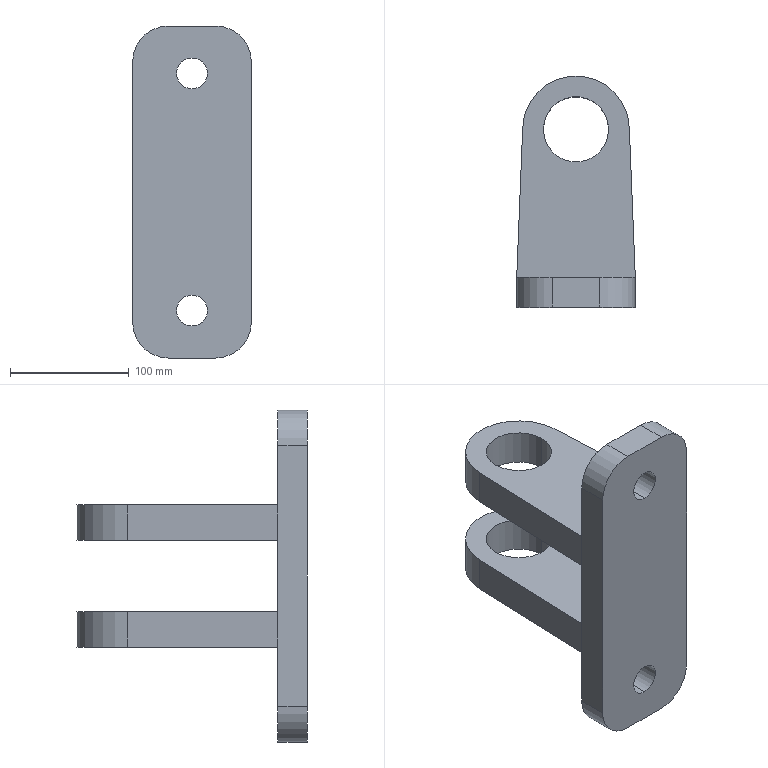Part | SolidWorks | features ICE 3, Extrusion 1, Fillet 1, MirrorPattern 1 | 1 solid | 30 faces | box 100 x 195 x 280 mm | volume 1415210 mm3 | plane 16 | cylinder 14 | commonest cylinder face diameters 26 x4 55 x4 60 x4 90 x2
STEP:
#1=CARTESIAN_POINT('',(0.,25.,87.));
#2=VERTEX_POINT('',#1);
#3=CARTESIAN_POINT('',(0.,25.,113.));
#4=VERTEX_POINT('',#3);
#5=CARTESIAN_POINT('',(0.,25.,100.));
#6=DIRECTION('',(0.,1.,0.));
#7=DIRECTION('',(0.,0.,-1.));
#8=AXIS2_PLACEMENT_3D('',#5,#6,#7);
#9=CIRCLE('',#8,13.);
#10=EDGE_CURVE('',#2,#4,#9,.T.);
#11=ORIENTED_EDGE('',*,*,#10,.T.);
#12=CARTESIAN_POINT('',(0.,0.,113.));
#13=VERTEX_POINT('',#12);
#14=CARTESIAN_POINT('',(0.,322.321,113.));
#15=DIRECTION('',(0.,-1.,0.));
#16=VECTOR('',#15,1000.);
#17=LINE('',#14,#16);
#18=EDGE_CURVE('',#4,#13,#17,.T.);
#19=ORIENTED_EDGE('',*,*,#18,.T.);
#20=CARTESIAN_POINT('',(0.,0.,87.));
#21=VERTEX_POINT('',#20);
#22=CARTESIAN_POINT('',(0.,0.,100.));
#23=DIRECTION('',(0.,-1.,0.));
#24=DIRECTION('',(0.,0.,1.));
#25=AXIS2_PLACEMENT_3D('',#22,#23,#24);
#26=CIRCLE('',#25,13.);
#27=EDGE_CURVE('',#13,#21,#26,.T.);
#28=ORIENTED_EDGE('',*,*,#27,.T.);
#29=CARTESIAN_POINT('',(0.,322.321,87.));
#30=DIRECTION('',(0.,-1.,0.));
#31=VECTOR('',#30,1000.);
#32=LINE('',#29,#31);
#33=EDGE_CURVE('',#2,#21,#32,.T.);
#34=ORIENTED_EDGE('',*,*,#33,.F.);
#35=EDGE_LOOP('',(#11,#19,#28,#34));
#36=FACE_OUTER_BOUND('',#35,.T.);
#37=CARTESIAN_POINT('',(0.,322.321,100.));
#38=DIRECTION('',(0.,-1.,0.));
#39=DIRECTION('',(0.,0.,-1.));
#40=AXIS2_PLACEMENT_3D('',#37,#38,#39);
#41=CYLINDRICAL_SURFACE('',#40,13.);
#42=ADVANCED_FACE('',(#36),#41,.F.);
#43=CARTESIAN_POINT('',(0.,25.,-113.));
#44=VERTEX_POINT('',#43);
#45=CARTESIAN_POINT('',(0.,25.,-87.));
#46=VERTEX_POINT('',#45);
#47=CARTESIAN_POINT('',(0.,25.,-100.));
#48=DIRECTION('',(0.,1.,0.));
#49=DIRECTION('',(0.,0.,-1.));
#50=AXIS2_PLACEMENT_3D('',#47,#48,#49);
#51=CIRCLE('',#50,13.);
#52=EDGE_CURVE('',#44,#46,#51,.T.);
#53=ORIENTED_EDGE('',*,*,#52,.T.);
#54=CARTESIAN_POINT('',(0.,0.,-87.));
#55=VERTEX_POINT('',#54);
#56=CARTESIAN_POINT('',(0.,322.321,-87.));
#57=DIRECTION('',(0.,-1.,0.));
#58=VECTOR('',#57,1000.);
#59=LINE('',#56,#58);
#60=EDGE_CURVE('',#46,#55,#59,.T.);
#61=ORIENTED_EDGE('',*,*,#60,.T.);
#62=CARTESIAN_POINT('',(0.,0.,-113.));
#63=VERTEX_POINT('',#62);
#64=CARTESIAN_POINT('',(0.,0.,-100.));
#65=DIRECTION('',(0.,-1.,0.));
#66=DIRECTION('',(0.,0.,-1.));
#67=AXIS2_PLACEMENT_3D('',#64,#65,#66);
#68=CIRCLE('',#67,13.);
#69=EDGE_CURVE('',#55,#63,#68,.T.);
#70=ORIENTED_EDGE('',*,*,#69,.T.);
#71=CARTESIAN_POINT('',(0.,322.321,-113.));
#72=DIRECTION('',(0.,-1.,0.));
#73=VECTOR('',#72,1000.);
#74=LINE('',#71,#73);
#75=EDGE_CURVE('',#44,#63,#74,.T.);
#76=ORIENTED_EDGE('',*,*,#75,.F.);
#77=EDGE_LOOP('',(#53,#61,#70,#76));
#78=FACE_OUTER_BOUND('',#77,.T.);
#79=CARTESIAN_POINT('',(0.,322.321,-100.));
#80=DIRECTION('',(0.,-1.,0.));
#81=DIRECTION('',(0.,0.,-1.));
#82=AXIS2_PLACEMENT_3D('',#79,#80,#81);
#83=CYLINDRICAL_SURFACE('',#82,13.);
#84=ADVANCED_FACE('',(#78),#83,.F.);
#85=CARTESIAN_POINT('',(-27.5,150.,-30.));
#86=VERTEX_POINT('',#85);
#87=CARTESIAN_POINT('',(27.5,150.,-30.));
#88=VERTEX_POINT('',#87);
#89=CARTESIAN_POINT('',(0.,150.,-30.));
#90=DIRECTION('',(0.,0.,1.));
#91=DIRECTION('',(1.,0.,0.));
#92=AXIS2_PLACEMENT_3D('',#89,#90,#91);
#93=CIRCLE('',#92,27.5);
#94=EDGE_CURVE('',#86,#88,#93,.T.);
#95=ORIENTED_EDGE('',*,*,#94,.T.);
#96=CARTESIAN_POINT('',(27.5,150.,-60.));
#97=VERTEX_POINT('',#96);
#98=CARTESIAN_POINT('',(27.5,150.,-30.));
#99=DIRECTION('',(0.,0.,-1.));
#100=VECTOR('',#99,1000.);
#101=LINE('',#98,#100);
#102=EDGE_CURVE('',#88,#97,#101,.T.);
#103=ORIENTED_EDGE('',*,*,#102,.T.);
#104=CARTESIAN_POINT('',(-27.5,150.,-60.));
#105=VERTEX_POINT('',#104);
#106=CARTESIAN_POINT('',(0.,150.,-60.));
#107=DIRECTION('',(0.,0.,1.));
#108=DIRECTION('',(1.,0.,0.));
#109=AXIS2_PLACEMENT_3D('',#106,#107,#108);
#110=CIRCLE('',#109,27.5);
#111=EDGE_CURVE('',#105,#97,#110,.T.);
#112=ORIENTED_EDGE('',*,*,#111,.F.);
#113=CARTESIAN_POINT('',(-27.5,150.,-30.));
#114=DIRECTION('',(0.,0.,-1.));
#115=VECTOR('',#114,1000.);
#116=LINE('',#113,#115);
#117=EDGE_CURVE('',#86,#105,#116,.T.);
#118=ORIENTED_EDGE('',*,*,#117,.F.);
#119=EDGE_LOOP('',(#95,#103,#112,#118));
#120=FACE_OUTER_BOUND('',#119,.T.);
#121=CARTESIAN_POINT('',(0.,150.,-30.));
#122=DIRECTION('',(0.,0.,-1.));
#123=DIRECTION('',(-1.,0.,0.));
#124=AXIS2_PLACEMENT_3D('',#121,#122,#123);
#125=CYLINDRICAL_SURFACE('',#124,27.5);
#126=ADVANCED_FACE('',(#120),#125,.F.);
#127=CARTESIAN_POINT('',(-27.5,150.,30.));
#128=VERTEX_POINT('',#127);
#129=CARTESIAN_POINT('',(27.5,150.,30.));
#130=VERTEX_POINT('',#129);
#131=CARTESIAN_POINT('',(0.,150.,30.));
#132=DIRECTION('',(0.,0.,1.));
#133=DIRECTION('',(1.,0.,0.));
#134=AXIS2_PLACEMENT_3D('',#131,#132,#133);
#135=CIRCLE('',#134,27.5);
#136=EDGE_CURVE('',#128,#130,#135,.T.);
#137=ORIENTED_EDGE('',*,*,#136,.F.);
#138=CARTESIAN_POINT('',(-27.5,150.,60.));
#139=VERTEX_POINT('',#138);
#140=CARTESIAN_POINT('',(-27.5,150.,30.));
#141=DIRECTION('',(0.,0.,1.));
#142=VECTOR('',#141,1000.);
#143=LINE('',#140,#142);
#144=EDGE_CURVE('',#128,#139,#143,.T.);
#145=ORIENTED_EDGE('',*,*,#144,.T.);
#146=CARTESIAN_POINT('',(27.5,150.,60.));
#147=VERTEX_POINT('',#146);
#148=CARTESIAN_POINT('',(0.,150.,60.));
#149=DIRECTION('',(0.,0.,1.));
#150=DIRECTION('',(1.,0.,0.));
#151=AXIS2_PLACEMENT_3D('',#148,#149,#150);
#152=CIRCLE('',#151,27.5);
#153=EDGE_CURVE('',#139,#147,#152,.T.);
#154=ORIENTED_EDGE('',*,*,#153,.T.);
#155=CARTESIAN_POINT('',(27.5,150.,30.));
#156=DIRECTION('',(0.,0.,1.));
#157=VECTOR('',#156,1000.);
#158=LINE('',#155,#157);
#159=EDGE_CURVE('',#130,#147,#158,.T.);
#160=ORIENTED_EDGE('',*,*,#159,.F.);
#161=EDGE_LOOP('',(#137,#145,#154,#160));
#162=FACE_OUTER_BOUND('',#161,.T.);
#163=CARTESIAN_POINT('',(0.,150.,30.));
#164=DIRECTION('',(0.,0.,1.));
#165=DIRECTION('',(1.,0.,0.));
#166=AXIS2_PLACEMENT_3D('',#163,#164,#165);
#167=CYLINDRICAL_SURFACE('',#166,27.5);
#168=ADVANCED_FACE('',(#162),#167,.F.);
#169=CARTESIAN_POINT('',(0.,150.,60.));
#170=DIRECTION('',(0.,0.,1.));
#171=DIRECTION('',(1.,0.,0.));
#172=AXIS2_PLACEMENT_3D('',#169,#170,#171);
#173=CIRCLE('',#172,27.5);
#174=EDGE_CURVE('',#147,#139,#173,.T.);
#175=ORIENTED_EDGE('',*,*,#174,.F.);
#176=ORIENTED_EDGE('',*,*,#153,.F.);
#177=EDGE_LOOP('',(#175,#176));
#178=FACE_BOUND('',#177,.T.);
#179=CARTESIAN_POINT('',(50.,25.,60.));
#180=VERTEX_POINT('',#179);
#181=CARTESIAN_POINT('',(-50.,25.,60.));
#182=VERTEX_POINT('',#181);
#183=CARTESIAN_POINT('',(-7.5,25.,60.));
#184=DIRECTION('',(-1.,0.,0.));
#185=VECTOR('',#184,1000.);
#186=LINE('',#183,#185);
#187=EDGE_CURVE('',#180,#182,#186,.T.);
#188=ORIENTED_EDGE('',*,*,#187,.F.);
#189=CARTESIAN_POINT('',(44.965,151.786,60.));
#190=VERTEX_POINT('',#189);
#191=CARTESIAN_POINT('',(44.965,151.786,60.));
#192=DIRECTION('',(-0.03968,0.9992,0.));
#193=VECTOR('',#192,1000.);
#194=LINE('',#191,#193);
#195=EDGE_CURVE('',#180,#190,#194,.T.);
#196=ORIENTED_EDGE('',*,*,#195,.T.);
#197=CARTESIAN_POINT('',(-44.965,151.786,60.));
#198=VERTEX_POINT('',#197);
#199=CARTESIAN_POINT('',(0.,150.,60.));
#200=DIRECTION('',(0.,0.,1.));
#201=DIRECTION('',(1.,0.,0.));
#202=AXIS2_PLACEMENT_3D('',#199,#200,#201);
#203=CIRCLE('',#202,45.);
#204=EDGE_CURVE('',#190,#198,#203,.T.);
#205=ORIENTED_EDGE('',*,*,#204,.T.);
#206=CARTESIAN_POINT('',(-44.965,151.786,60.));
#207=DIRECTION('',(-0.03968,-0.9992,0.));
#208=VECTOR('',#207,1000.);
#209=LINE('',#206,#208);
#210=EDGE_CURVE('',#198,#182,#209,.T.);
#211=ORIENTED_EDGE('',*,*,#210,.T.);
#212=EDGE_LOOP('',(#188,#196,#205,#211));
#213=FACE_OUTER_BOUND('',#212,.T.);
#214=CARTESIAN_POINT('',(-50.,25.,60.));
#215=DIRECTION('',(0.,0.,-1.));
#216=DIRECTION('',(-1.,0.,0.));
#217=AXIS2_PLACEMENT_3D('',#214,#215,#216);
#218=PLANE('',#217);
#219=ADVANCED_FACE('',(#178,#213),#218,.F.);
#220=ORIENTED_EDGE('',*,*,#111,.T.);
#221=CARTESIAN_POINT('',(0.,150.,-60.));
#222=DIRECTION('',(0.,0.,1.));
#223=DIRECTION('',(1.,0.,0.));
#224=AXIS2_PLACEMENT_3D('',#221,#222,#223);
#225=CIRCLE('',#224,27.5);
#226=EDGE_CURVE('',#97,#105,#225,.T.);
#227=ORIENTED_EDGE('',*,*,#226,.T.);
#228=EDGE_LOOP('',(#220,#227));
#229=FACE_BOUND('',#228,.T.);
#230=CARTESIAN_POINT('',(50.,25.,-60.));
#231=VERTEX_POINT('',#230);
#232=CARTESIAN_POINT('',(-50.,25.,-60.));
#233=VERTEX_POINT('',#232);
#234=CARTESIAN_POINT('',(-7.5,25.,-60.));
#235=DIRECTION('',(-1.,0.,0.));
#236=VECTOR('',#235,1000.);
#237=LINE('',#234,#236);
#238=EDGE_CURVE('',#231,#233,#237,.T.);
#239=ORIENTED_EDGE('',*,*,#238,.T.);
#240=CARTESIAN_POINT('',(-44.965,151.786,-60.));
#241=VERTEX_POINT('',#240);
#242=CARTESIAN_POINT('',(-44.965,151.786,-60.));
#243=DIRECTION('',(-0.03968,-0.9992,0.));
#244=VECTOR('',#243,1000.);
#245=LINE('',#242,#244);
#246=EDGE_CURVE('',#241,#233,#245,.T.);
#247=ORIENTED_EDGE('',*,*,#246,.F.);
#248=CARTESIAN_POINT('',(44.965,151.786,-60.));
#249=VERTEX_POINT('',#248);
#250=CARTESIAN_POINT('',(0.,150.,-60.));
#251=DIRECTION('',(0.,0.,1.));
#252=DIRECTION('',(1.,0.,0.));
#253=AXIS2_PLACEMENT_3D('',#250,#251,#252);
#254=CIRCLE('',#253,45.);
#255=EDGE_CURVE('',#249,#241,#254,.T.);
#256=ORIENTED_EDGE('',*,*,#255,.F.);
#257=CARTESIAN_POINT('',(44.965,151.786,-60.));
#258=DIRECTION('',(-0.03968,0.9992,0.));
#259=VECTOR('',#258,1000.);
#260=LINE('',#257,#259);
#261=EDGE_CURVE('',#231,#249,#260,.T.);
#262=ORIENTED_EDGE('',*,*,#261,.F.);
#263=EDGE_LOOP('',(#239,#247,#256,#262));
#264=FACE_OUTER_BOUND('',#263,.T.);
#265=CARTESIAN_POINT('',(-50.,25.,-60.));
#266=DIRECTION('',(0.,0.,1.));
#267=DIRECTION('',(1.,0.,0.));
#268=AXIS2_PLACEMENT_3D('',#265,#266,#267);
#269=PLANE('',#268);
#270=ADVANCED_FACE('',(#229,#264),#269,.F.);
#271=CARTESIAN_POINT('',(-50.,25.,-30.));
#272=VERTEX_POINT('',#271);
#273=CARTESIAN_POINT('',(50.,25.,-30.));
#274=VERTEX_POINT('',#273);
#275=CARTESIAN_POINT('',(-50.,25.,-30.));
#276=DIRECTION('',(1.,0.,0.));
#277=VECTOR('',#276,1000.);
#278=LINE('',#275,#277);
#279=EDGE_CURVE('',#272,#274,#278,.T.);
#280=ORIENTED_EDGE('',*,*,#279,.F.);
#281=CARTESIAN_POINT('',(-50.,25.,30.));
#282=VERTEX_POINT('',#281);
#283=CARTESIAN_POINT('',(-50.,25.,60.));
#284=DIRECTION('',(0.,0.,1.));
#285=VECTOR('',#284,1000.);
#286=LINE('',#283,#285);
#287=EDGE_CURVE('',#272,#282,#286,.T.);
#288=ORIENTED_EDGE('',*,*,#287,.T.);
#289=CARTESIAN_POINT('',(50.,25.,30.));
#290=VERTEX_POINT('',#289);
#291=CARTESIAN_POINT('',(-50.,25.,30.));
#292=DIRECTION('',(1.,0.,0.));
#293=VECTOR('',#292,1000.);
#294=LINE('',#291,#293);
#295=EDGE_CURVE('',#282,#290,#294,.T.);
#296=ORIENTED_EDGE('',*,*,#295,.T.);
#297=CARTESIAN_POINT('',(50.,25.,60.));
#298=DIRECTION('',(0.,0.,-1.));
#299=VECTOR('',#298,1000.);
#300=LINE('',#297,#299);
#301=EDGE_CURVE('',#290,#274,#300,.T.);
#302=ORIENTED_EDGE('',*,*,#301,.T.);
#303=EDGE_LOOP('',(#280,#288,#296,#302));
#304=FACE_OUTER_BOUND('',#303,.T.);
#305=CARTESIAN_POINT('',(0.,25.,0.));
#306=DIRECTION('',(0.,-1.,0.));
#307=DIRECTION('',(0.,0.,-1.));
#308=AXIS2_PLACEMENT_3D('',#305,#306,#307);
#309=PLANE('',#308);
#310=ADVANCED_FACE('',(#304),#309,.F.);
#311=CARTESIAN_POINT('',(50.,25.,110.));
#312=VERTEX_POINT('',#311);
#313=CARTESIAN_POINT('',(50.,25.,-140.));
#314=DIRECTION('',(0.,0.,-1.));
#315=VECTOR('',#314,1000.);
#316=LINE('',#313,#315);
#317=EDGE_CURVE('',#312,#180,#316,.T.);
#318=ORIENTED_EDGE('',*,*,#317,.F.);
#319=CARTESIAN_POINT('',(50.,0.,110.));
#320=VERTEX_POINT('',#319);
#321=CARTESIAN_POINT('',(50.,0.,110.));
#322=DIRECTION('',(0.,-1.,0.));
#323=VECTOR('',#322,1000.);
#324=LINE('',#321,#323);
#325=EDGE_CURVE('',#312,#320,#324,.T.);
#326=ORIENTED_EDGE('',*,*,#325,.T.);
#327=CARTESIAN_POINT('',(50.,0.,-110.));
#328=VERTEX_POINT('',#327);
#329=CARTESIAN_POINT('',(50.,0.,60.));
#330=DIRECTION('',(0.,0.,-1.));
#331=VECTOR('',#330,1000.);
#332=LINE('',#329,#331);
#333=EDGE_CURVE('',#320,#328,#332,.T.);
#334=ORIENTED_EDGE('',*,*,#333,.T.);
#335=CARTESIAN_POINT('',(50.,25.,-110.));
#336=VERTEX_POINT('',#335);
#337=CARTESIAN_POINT('',(50.,25.,-110.));
#338=DIRECTION('',(0.,1.,0.));
#339=VECTOR('',#338,1000.);
#340=LINE('',#337,#339);
#341=EDGE_CURVE('',#328,#336,#340,.T.);
#342=ORIENTED_EDGE('',*,*,#341,.T.);
#343=CARTESIAN_POINT('',(50.,25.,-140.));
#344=DIRECTION('',(0.,0.,-1.));
#345=VECTOR('',#344,1000.);
#346=LINE('',#343,#345);
#347=EDGE_CURVE('',#231,#336,#346,.T.);
#348=ORIENTED_EDGE('',*,*,#347,.F.);
#349=CARTESIAN_POINT('',(50.,25.,-30.));
#350=DIRECTION('',(0.,0.,-1.));
#351=VECTOR('',#350,1000.);
#352=LINE('',#349,#351);
#353=EDGE_CURVE('',#274,#231,#352,.T.);
#354=ORIENTED_EDGE('',*,*,#353,.F.);
#355=ORIENTED_EDGE('',*,*,#301,.F.);
#356=CARTESIAN_POINT('',(50.,25.,60.));
#357=DIRECTION('',(0.,0.,-1.));
#358=VECTOR('',#357,1000.);
#359=LINE('',#356,#358);
#360=EDGE_CURVE('',#180,#290,#359,.T.);
#361=ORIENTED_EDGE('',*,*,#360,.F.);
#362=EDGE_LOOP('',(#318,#326,#334,#342,#348,#354,#355,#361));
#363=FACE_OUTER_BOUND('',#362,.T.);
#364=CARTESIAN_POINT('',(50.,25.,60.));
#365=DIRECTION('',(-1.,0.,0.));
#366=DIRECTION('',(0.,0.,1.));
#367=AXIS2_PLACEMENT_3D('',#364,#365,#366);
#368=PLANE('',#367);
#369=ADVANCED_FACE('',(#363),#368,.F.);
#370=CARTESIAN_POINT('',(-50.,0.,-110.));
#371=VERTEX_POINT('',#370);
#372=CARTESIAN_POINT('',(-50.,0.,110.));
#373=VERTEX_POINT('',#372);
#374=CARTESIAN_POINT('',(-50.,0.,60.));
#375=DIRECTION('',(0.,0.,1.));
#376=VECTOR('',#375,1000.);
#377=LINE('',#374,#376);
#378=EDGE_CURVE('',#371,#373,#377,.T.);
#379=ORIENTED_EDGE('',*,*,#378,.T.);
#380=CARTESIAN_POINT('',(-50.,25.,110.));
#381=VERTEX_POINT('',#380);
#382=CARTESIAN_POINT('',(-50.,25.,110.));
#383=DIRECTION('',(0.,1.,0.));
#384=VECTOR('',#383,1000.);
#385=LINE('',#382,#384);
#386=EDGE_CURVE('',#373,#381,#385,.T.);
#387=ORIENTED_EDGE('',*,*,#386,.T.);
#388=CARTESIAN_POINT('',(-50.,25.,-140.));
#389=DIRECTION('',(0.,0.,1.));
#390=VECTOR('',#389,1000.);
#391=LINE('',#388,#390);
#392=EDGE_CURVE('',#182,#381,#391,.T.);
#393=ORIENTED_EDGE('',*,*,#392,.F.);
#394=CARTESIAN_POINT('',(-50.,25.,30.));
#395=DIRECTION('',(0.,0.,1.));
#396=VECTOR('',#395,1000.);
#397=LINE('',#394,#396);
#398=EDGE_CURVE('',#282,#182,#397,.T.);
#399=ORIENTED_EDGE('',*,*,#398,.F.);
#400=ORIENTED_EDGE('',*,*,#287,.F.);
#401=CARTESIAN_POINT('',(-50.,25.,60.));
#402=DIRECTION('',(0.,0.,1.));
#403=VECTOR('',#402,1000.);
#404=LINE('',#401,#403);
#405=EDGE_CURVE('',#233,#272,#404,.T.);
#406=ORIENTED_EDGE('',*,*,#405,.F.);
#407=CARTESIAN_POINT('',(-50.,25.,-110.));
#408=VERTEX_POINT('',#407);
#409=CARTESIAN_POINT('',(-50.,25.,-140.));
#410=DIRECTION('',(0.,0.,1.));
#411=VECTOR('',#410,1000.);
#412=LINE('',#409,#411);
#413=EDGE_CURVE('',#408,#233,#412,.T.);
#414=ORIENTED_EDGE('',*,*,#413,.F.);
#415=CARTESIAN_POINT('',(-50.,0.,-110.));
#416=DIRECTION('',(0.,-1.,0.));
#417=VECTOR('',#416,1000.);
#418=LINE('',#415,#417);
#419=EDGE_CURVE('',#408,#371,#418,.T.);
#420=ORIENTED_EDGE('',*,*,#419,.T.);
#421=EDGE_LOOP('',(#379,#387,#393,#399,#400,#406,#414,#420));
#422=FACE_OUTER_BOUND('',#421,.T.);
#423=CARTESIAN_POINT('',(-50.,25.,60.));
#424=DIRECTION('',(1.,0.,0.));
#425=DIRECTION('',(0.,0.,-1.));
#426=AXIS2_PLACEMENT_3D('',#423,#424,#425);
#427=PLANE('',#426);
#428=ADVANCED_FACE('',(#422),#427,.F.);
#429=ORIENTED_EDGE('',*,*,#333,.F.);
#430=CARTESIAN_POINT('',(20.,0.,140.));
#431=VERTEX_POINT('',#430);
#432=CARTESIAN_POINT('',(20.,0.,110.));
#433=DIRECTION('',(0.,-1.,0.));
#434=DIRECTION('',(0.,0.,-1.));
#435=AXIS2_PLACEMENT_3D('',#432,#433,#434);
#436=CIRCLE('',#435,30.);
#437=EDGE_CURVE('',#320,#431,#436,.T.);
#438=ORIENTED_EDGE('',*,*,#437,.T.);
#439=CARTESIAN_POINT('',(-20.,0.,140.));
#440=VERTEX_POINT('',#439);
#441=CARTESIAN_POINT('',(50.,0.,140.));
#442=DIRECTION('',(-1.,0.,0.));
#443=VECTOR('',#442,1000.);
#444=LINE('',#441,#443);
#445=EDGE_CURVE('',#431,#440,#444,.T.);
#446=ORIENTED_EDGE('',*,*,#445,.T.);
#447=CARTESIAN_POINT('',(-20.,0.,110.));
#448=DIRECTION('',(0.,-1.,0.));
#449=DIRECTION('',(0.,0.,-1.));
#450=AXIS2_PLACEMENT_3D('',#447,#448,#449);
#451=CIRCLE('',#450,30.);
#452=EDGE_CURVE('',#440,#373,#451,.T.);
#453=ORIENTED_EDGE('',*,*,#452,.T.);
#454=ORIENTED_EDGE('',*,*,#378,.F.);
#455=CARTESIAN_POINT('',(-20.,0.,-140.));
#456=VERTEX_POINT('',#455);
#457=CARTESIAN_POINT('',(-20.,0.,-110.));
#458=DIRECTION('',(0.,-1.,0.));
#459=DIRECTION('',(0.,0.,-1.));
#460=AXIS2_PLACEMENT_3D('',#457,#458,#459);
#461=CIRCLE('',#460,30.);
#462=EDGE_CURVE('',#371,#456,#461,.T.);
#463=ORIENTED_EDGE('',*,*,#462,.T.);
#464=CARTESIAN_POINT('',(20.,0.,-140.));
#465=VERTEX_POINT('',#464);
#466=CARTESIAN_POINT('',(50.,0.,-140.));
#467=DIRECTION('',(1.,0.,0.));
#468=VECTOR('',#467,1000.);
#469=LINE('',#466,#468);
#470=EDGE_CURVE('',#456,#465,#469,.T.);
#471=ORIENTED_EDGE('',*,*,#470,.T.);
#472=CARTESIAN_POINT('',(20.,0.,-110.));
#473=DIRECTION('',(0.,-1.,0.));
#474=DIRECTION('',(0.,0.,-1.));
#475=AXIS2_PLACEMENT_3D('',#472,#473,#474);
#476=CIRCLE('',#475,30.);
#477=EDGE_CURVE('',#465,#328,#476,.T.);
#478=ORIENTED_EDGE('',*,*,#477,.T.);
#479=EDGE_LOOP('',(#429,#438,#446,#453,#454,#463,#471,#478));
#480=FACE_OUTER_BOUND('',#479,.T.);
#481=CARTESIAN_POINT('',(0.,0.,-100.));
#482=DIRECTION('',(0.,-1.,0.));
#483=DIRECTION('',(0.,0.,-1.));
#484=AXIS2_PLACEMENT_3D('',#481,#482,#483);
#485=CIRCLE('',#484,13.);
#486=EDGE_CURVE('',#63,#55,#485,.T.);
#487=ORIENTED_EDGE('',*,*,#486,.F.);
#488=ORIENTED_EDGE('',*,*,#69,.F.);
#489=EDGE_LOOP('',(#487,#488));
#490=FACE_BOUND('',#489,.T.);
#491=CARTESIAN_POINT('',(0.,0.,100.));
#492=DIRECTION('',(0.,-1.,0.));
#493=DIRECTION('',(0.,0.,1.));
#494=AXIS2_PLACEMENT_3D('',#491,#492,#493);
#495=CIRCLE('',#494,13.);
#496=EDGE_CURVE('',#21,#13,#495,.T.);
#497=ORIENTED_EDGE('',*,*,#496,.F.);
#498=ORIENTED_EDGE('',*,*,#27,.F.);
#499=EDGE_LOOP('',(#497,#498));
#500=FACE_BOUND('',#499,.T.);
#501=CARTESIAN_POINT('',(0.,0.,0.));
#502=DIRECTION('',(0.,-1.,0.));
#503=DIRECTION('',(0.,0.,-1.));
#504=AXIS2_PLACEMENT_3D('',#501,#502,#503);
#505=PLANE('',#504);
#506=ADVANCED_FACE('',(#480,#490,#500),#505,.T.);
#507=ORIENTED_EDGE('',*,*,#204,.F.);
#508=CARTESIAN_POINT('',(44.965,151.786,30.));
#509=VERTEX_POINT('',#508);
#510=CARTESIAN_POINT('',(44.965,151.786,30.));
#511=DIRECTION('',(0.,0.,1.));
#512=VECTOR('',#511,1000.);
#513=LINE('',#510,#512);
#514=EDGE_CURVE('',#509,#190,#513,.T.);
#515=ORIENTED_EDGE('',*,*,#514,.F.);
#516=CARTESIAN_POINT('',(-44.965,151.786,30.));
#517=VERTEX_POINT('',#516);
#518=CARTESIAN_POINT('',(0.,150.,30.));
#519=DIRECTION('',(0.,0.,1.));
#520=DIRECTION('',(1.,0.,0.));
#521=AXIS2_PLACEMENT_3D('',#518,#519,#520);
#522=CIRCLE('',#521,45.);
#523=EDGE_CURVE('',#509,#517,#522,.T.);
#524=ORIENTED_EDGE('',*,*,#523,.T.);
#525=CARTESIAN_POINT('',(-44.965,151.786,30.));
#526=DIRECTION('',(0.,0.,1.));
#527=VECTOR('',#526,1000.);
#528=LINE('',#525,#527);
#529=EDGE_CURVE('',#517,#198,#528,.T.);
#530=ORIENTED_EDGE('',*,*,#529,.T.);
#531=EDGE_LOOP('',(#507,#515,#524,#530));
#532=FACE_OUTER_BOUND('',#531,.T.);
#533=CARTESIAN_POINT('',(0.,150.,30.));
#534=DIRECTION('',(0.,0.,1.));
#535=DIRECTION('',(1.,0.,0.));
#536=AXIS2_PLACEMENT_3D('',#533,#534,#535);
#537=CYLINDRICAL_SURFACE('',#536,45.);
#538=ADVANCED_FACE('',(#532),#537,.T.);
#539=ORIENTED_EDGE('',*,*,#195,.F.);
#540=ORIENTED_EDGE('',*,*,#360,.T.);
#541=CARTESIAN_POINT('',(44.965,151.786,30.));
#542=DIRECTION('',(-0.03968,0.9992,0.));
#543=VECTOR('',#542,1000.);
#544=LINE('',#541,#543);
#545=EDGE_CURVE('',#290,#509,#544,.T.);
#546=ORIENTED_EDGE('',*,*,#545,.T.);
#547=ORIENTED_EDGE('',*,*,#514,.T.);
#548=EDGE_LOOP('',(#539,#540,#546,#547));
#549=FACE_OUTER_BOUND('',#548,.T.);
#550=CARTESIAN_POINT('',(44.965,151.786,30.));
#551=DIRECTION('',(0.9992,0.03968,0.));
#552=DIRECTION('',(-0.03968,0.9992,0.));
#553=AXIS2_PLACEMENT_3D('',#550,#551,#552);
#554=PLANE('',#553);
#555=ADVANCED_FACE('',(#549),#554,.T.);
#556=ORIENTED_EDGE('',*,*,#210,.F.);
#557=ORIENTED_EDGE('',*,*,#529,.F.);
#558=CARTESIAN_POINT('',(-44.965,151.786,30.));
#559=DIRECTION('',(-0.03968,-0.9992,0.));
#560=VECTOR('',#559,1000.);
#561=LINE('',#558,#560);
#562=EDGE_CURVE('',#517,#282,#561,.T.);
#563=ORIENTED_EDGE('',*,*,#562,.T.);
#564=ORIENTED_EDGE('',*,*,#398,.T.);
#565=EDGE_LOOP('',(#556,#557,#563,#564));
#566=FACE_OUTER_BOUND('',#565,.T.);
#567=CARTESIAN_POINT('',(-44.965,151.786,30.));
#568=DIRECTION('',(-0.9992,0.03968,0.));
#569=DIRECTION('',(-0.03968,-0.9992,0.));
#570=AXIS2_PLACEMENT_3D('',#567,#568,#569);
#571=PLANE('',#570);
#572=ADVANCED_FACE('',(#566),#571,.T.);
#573=CARTESIAN_POINT('',(0.,150.,30.));
#574=DIRECTION('',(0.,0.,1.));
#575=DIRECTION('',(1.,0.,0.));
#576=AXIS2_PLACEMENT_3D('',#573,#574,#575);
#577=CIRCLE('',#576,27.5);
#578=EDGE_CURVE('',#130,#128,#577,.T.);
#579=ORIENTED_EDGE('',*,*,#578,.T.);
#580=ORIENTED_EDGE('',*,*,#136,.T.);
#581=EDGE_LOOP('',(#579,#580));
#582=FACE_BOUND('',#581,.T.);
#583=ORIENTED_EDGE('',*,*,#523,.F.);
#584=ORIENTED_EDGE('',*,*,#545,.F.);
#585=ORIENTED_EDGE('',*,*,#295,.F.);
#586=ORIENTED_EDGE('',*,*,#562,.F.);
#587=EDGE_LOOP('',(#583,#584,#585,#586));
#588=FACE_OUTER_BOUND('',#587,.T.);
#589=CARTESIAN_POINT('',(0.,150.,30.));
#590=DIRECTION('',(0.,0.,1.));
#591=DIRECTION('',(1.,0.,0.));
#592=AXIS2_PLACEMENT_3D('',#589,#590,#591);
#593=PLANE('',#592);
#594=ADVANCED_FACE('',(#582,#588),#593,.F.);
#595=ORIENTED_EDGE('',*,*,#144,.F.);
#596=ORIENTED_EDGE('',*,*,#578,.F.);
#597=ORIENTED_EDGE('',*,*,#159,.T.);
#598=ORIENTED_EDGE('',*,*,#174,.T.);
#599=EDGE_LOOP('',(#595,#596,#597,#598));
#600=FACE_OUTER_BOUND('',#599,.T.);
#601=CARTESIAN_POINT('',(0.,150.,30.));
#602=DIRECTION('',(0.,0.,1.));
#603=DIRECTION('',(1.,0.,0.));
#604=AXIS2_PLACEMENT_3D('',#601,#602,#603);
#605=CYLINDRICAL_SURFACE('',#604,27.5);
#606=ADVANCED_FACE('',(#600),#605,.F.);
#607=CARTESIAN_POINT('',(-20.,25.,140.));
#608=VERTEX_POINT('',#607);
#609=CARTESIAN_POINT('',(20.,25.,140.));
#610=VERTEX_POINT('',#609);
#611=CARTESIAN_POINT('',(50.,25.,140.));
#612=DIRECTION('',(1.,0.,0.));
#613=VECTOR('',#612,1000.);
#614=LINE('',#611,#613);
#615=EDGE_CURVE('',#608,#610,#614,.T.);
#616=ORIENTED_EDGE('',*,*,#615,.T.);
#617=CARTESIAN_POINT('',(20.,25.,110.));
#618=DIRECTION('',(0.,1.,0.));
#619=DIRECTION('',(0.,0.,-1.));
#620=AXIS2_PLACEMENT_3D('',#617,#618,#619);
#621=CIRCLE('',#620,30.);
#622=EDGE_CURVE('',#610,#312,#621,.T.);
#623=ORIENTED_EDGE('',*,*,#622,.T.);
#624=ORIENTED_EDGE('',*,*,#317,.T.);
#625=ORIENTED_EDGE('',*,*,#187,.T.);
#626=ORIENTED_EDGE('',*,*,#392,.T.);
#627=CARTESIAN_POINT('',(-20.,25.,110.));
#628=DIRECTION('',(0.,1.,0.));
#629=DIRECTION('',(0.,0.,-1.));
#630=AXIS2_PLACEMENT_3D('',#627,#628,#629);
#631=CIRCLE('',#630,30.);
#632=EDGE_CURVE('',#381,#608,#631,.T.);
#633=ORIENTED_EDGE('',*,*,#632,.T.);
#634=EDGE_LOOP('',(#616,#623,#624,#625,#626,#633));
#635=FACE_OUTER_BOUND('',#634,.T.);
#636=ORIENTED_EDGE('',*,*,#10,.F.);
#637=CARTESIAN_POINT('',(0.,25.,100.));
#638=DIRECTION('',(0.,1.,0.));
#639=DIRECTION('',(0.,0.,-1.));
#640=AXIS2_PLACEMENT_3D('',#637,#638,#639);
#641=CIRCLE('',#640,13.);
#642=EDGE_CURVE('',#4,#2,#641,.T.);
#643=ORIENTED_EDGE('',*,*,#642,.F.);
#644=EDGE_LOOP('',(#636,#643));
#645=FACE_BOUND('',#644,.T.);
#646=CARTESIAN_POINT('',(-7.5,25.,70.));
#647=DIRECTION('',(0.,-1.,0.));
#648=DIRECTION('',(0.,0.,-1.));
#649=AXIS2_PLACEMENT_3D('',#646,#647,#648);
#650=PLANE('',#649);
#651=ADVANCED_FACE('',(#635,#645),#650,.F.);
#652=CARTESIAN_POINT('',(44.965,151.786,-30.));
#653=VERTEX_POINT('',#652);
#654=CARTESIAN_POINT('',(-44.965,151.786,-30.));
#655=VERTEX_POINT('',#654);
#656=CARTESIAN_POINT('',(0.,150.,-30.));
#657=DIRECTION('',(0.,0.,1.));
#658=DIRECTION('',(1.,0.,0.));
#659=AXIS2_PLACEMENT_3D('',#656,#657,#658);
#660=CIRCLE('',#659,45.);
#661=EDGE_CURVE('',#653,#655,#660,.T.);
#662=ORIENTED_EDGE('',*,*,#661,.T.);
#663=CARTESIAN_POINT('',(-44.965,151.786,-30.));
#664=DIRECTION('',(-0.03968,-0.9992,0.));
#665=VECTOR('',#664,1000.);
#666=LINE('',#663,#665);
#667=EDGE_CURVE('',#655,#272,#666,.T.);
#668=ORIENTED_EDGE('',*,*,#667,.T.);
#669=ORIENTED_EDGE('',*,*,#279,.T.);
#670=CARTESIAN_POINT('',(44.965,151.786,-30.));
#671=DIRECTION('',(-0.03968,0.9992,0.));
#672=VECTOR('',#671,1000.);
#673=LINE('',#670,#672);
#674=EDGE_CURVE('',#274,#653,#673,.T.);
#675=ORIENTED_EDGE('',*,*,#674,.T.);
#676=EDGE_LOOP('',(#662,#668,#669,#675));
#677=FACE_OUTER_BOUND('',#676,.T.);
#678=ORIENTED_EDGE('',*,*,#94,.F.);
#679=CARTESIAN_POINT('',(0.,150.,-30.));
#680=DIRECTION('',(0.,0.,1.));
#681=DIRECTION('',(1.,0.,0.));
#682=AXIS2_PLACEMENT_3D('',#679,#680,#681);
#683=CIRCLE('',#682,27.5);
#684=EDGE_CURVE('',#88,#86,#683,.T.);
#685=ORIENTED_EDGE('',*,*,#684,.F.);
#686=EDGE_LOOP('',(#678,#685));
#687=FACE_BOUND('',#686,.T.);
#688=CARTESIAN_POINT('',(0.,150.,-30.));
#689=DIRECTION('',(0.,0.,-1.));
#690=DIRECTION('',(1.,0.,0.));
#691=AXIS2_PLACEMENT_3D('',#688,#689,#690);
#692=PLANE('',#691);
#693=ADVANCED_FACE('',(#677,#687),#692,.F.);
#694=ORIENTED_EDGE('',*,*,#255,.T.);
#695=CARTESIAN_POINT('',(-44.965,151.786,-30.));
#696=DIRECTION('',(0.,0.,-1.));
#697=VECTOR('',#696,1000.);
#698=LINE('',#695,#697);
#699=EDGE_CURVE('',#655,#241,#698,.T.);
#700=ORIENTED_EDGE('',*,*,#699,.F.);
#701=ORIENTED_EDGE('',*,*,#661,.F.);
#702=CARTESIAN_POINT('',(44.965,151.786,-30.));
#703=DIRECTION('',(0.,0.,-1.));
#704=VECTOR('',#703,1000.);
#705=LINE('',#702,#704);
#706=EDGE_CURVE('',#653,#249,#705,.T.);
#707=ORIENTED_EDGE('',*,*,#706,.T.);
#708=EDGE_LOOP('',(#694,#700,#701,#707));
#709=FACE_OUTER_BOUND('',#708,.T.);
#710=CARTESIAN_POINT('',(0.,150.,-30.));
#711=DIRECTION('',(0.,0.,-1.));
#712=DIRECTION('',(-1.,0.,0.));
#713=AXIS2_PLACEMENT_3D('',#710,#711,#712);
#714=CYLINDRICAL_SURFACE('',#713,45.);
#715=ADVANCED_FACE('',(#709),#714,.T.);
#716=ORIENTED_EDGE('',*,*,#246,.T.);
#717=ORIENTED_EDGE('',*,*,#405,.T.);
#718=ORIENTED_EDGE('',*,*,#667,.F.);
#719=ORIENTED_EDGE('',*,*,#699,.T.);
#720=EDGE_LOOP('',(#716,#717,#718,#719));
#721=FACE_OUTER_BOUND('',#720,.T.);
#722=CARTESIAN_POINT('',(-44.965,151.786,-30.));
#723=DIRECTION('',(0.9992,-0.03968,0.));
#724=DIRECTION('',(0.03968,0.9992,0.));
#725=AXIS2_PLACEMENT_3D('',#722,#723,#724);
#726=PLANE('',#725);
#727=ADVANCED_FACE('',(#721),#726,.F.);
#728=ORIENTED_EDGE('',*,*,#261,.T.);
#729=ORIENTED_EDGE('',*,*,#706,.F.);
#730=ORIENTED_EDGE('',*,*,#674,.F.);
#731=ORIENTED_EDGE('',*,*,#353,.T.);
#732=EDGE_LOOP('',(#728,#729,#730,#731));
#733=FACE_OUTER_BOUND('',#732,.T.);
#734=CARTESIAN_POINT('',(44.965,151.786,-30.));
#735=DIRECTION('',(-0.9992,-0.03968,0.));
#736=DIRECTION('',(0.03968,-0.9992,0.));
#737=AXIS2_PLACEMENT_3D('',#734,#735,#736);
#738=PLANE('',#737);
#739=ADVANCED_FACE('',(#733),#738,.F.);
#740=ORIENTED_EDGE('',*,*,#102,.F.);
#741=ORIENTED_EDGE('',*,*,#684,.T.);
#742=ORIENTED_EDGE('',*,*,#117,.T.);
#743=ORIENTED_EDGE('',*,*,#226,.F.);
#744=EDGE_LOOP('',(#740,#741,#742,#743));
#745=FACE_OUTER_BOUND('',#744,.T.);
#746=CARTESIAN_POINT('',(0.,150.,-30.));
#747=DIRECTION('',(0.,0.,-1.));
#748=DIRECTION('',(-1.,0.,0.));
#749=AXIS2_PLACEMENT_3D('',#746,#747,#748);
#750=CYLINDRICAL_SURFACE('',#749,27.5);
#751=ADVANCED_FACE('',(#745),#750,.F.);
#752=ORIENTED_EDGE('',*,*,#347,.T.);
#753=CARTESIAN_POINT('',(20.,25.,-140.));
#754=VERTEX_POINT('',#753);
#755=CARTESIAN_POINT('',(20.,25.,-110.));
#756=DIRECTION('',(0.,1.,0.));
#757=DIRECTION('',(0.,0.,1.));
#758=AXIS2_PLACEMENT_3D('',#755,#756,#757);
#759=CIRCLE('',#758,30.);
#760=EDGE_CURVE('',#336,#754,#759,.T.);
#761=ORIENTED_EDGE('',*,*,#760,.T.);
#762=CARTESIAN_POINT('',(-20.,25.,-140.));
#763=VERTEX_POINT('',#762);
#764=CARTESIAN_POINT('',(50.,25.,-140.));
#765=DIRECTION('',(-1.,0.,0.));
#766=VECTOR('',#765,1000.);
#767=LINE('',#764,#766);
#768=EDGE_CURVE('',#754,#763,#767,.T.);
#769=ORIENTED_EDGE('',*,*,#768,.T.);
#770=CARTESIAN_POINT('',(-20.,25.,-110.));
#771=DIRECTION('',(0.,1.,0.));
#772=DIRECTION('',(0.,0.,1.));
#773=AXIS2_PLACEMENT_3D('',#770,#771,#772);
#774=CIRCLE('',#773,30.);
#775=EDGE_CURVE('',#763,#408,#774,.T.);
#776=ORIENTED_EDGE('',*,*,#775,.T.);
#777=ORIENTED_EDGE('',*,*,#413,.T.);
#778=ORIENTED_EDGE('',*,*,#238,.F.);
#779=EDGE_LOOP('',(#752,#761,#769,#776,#777,#778));
#780=FACE_OUTER_BOUND('',#779,.T.);
#781=ORIENTED_EDGE('',*,*,#52,.F.);
#782=CARTESIAN_POINT('',(0.,25.,-100.));
#783=DIRECTION('',(0.,1.,0.));
#784=DIRECTION('',(0.,0.,-1.));
#785=AXIS2_PLACEMENT_3D('',#782,#783,#784);
#786=CIRCLE('',#785,13.);
#787=EDGE_CURVE('',#46,#44,#786,.T.);
#788=ORIENTED_EDGE('',*,*,#787,.F.);
#789=EDGE_LOOP('',(#781,#788));
#790=FACE_BOUND('',#789,.T.);
#791=CARTESIAN_POINT('',(-7.5,25.,-70.));
#792=DIRECTION('',(0.,1.,0.));
#793=DIRECTION('',(0.,0.,1.));
#794=AXIS2_PLACEMENT_3D('',#791,#792,#793);
#795=PLANE('',#794);
#796=ADVANCED_FACE('',(#780,#790),#795,.T.);
#797=ORIENTED_EDGE('',*,*,#768,.F.);
#798=CARTESIAN_POINT('',(20.,0.,-140.));
#799=DIRECTION('',(0.,-1.,0.));
#800=VECTOR('',#799,1000.);
#801=LINE('',#798,#800);
#802=EDGE_CURVE('',#754,#465,#801,.T.);
#803=ORIENTED_EDGE('',*,*,#802,.T.);
#804=ORIENTED_EDGE('',*,*,#470,.F.);
#805=CARTESIAN_POINT('',(-20.,25.,-140.));
#806=DIRECTION('',(0.,1.,0.));
#807=VECTOR('',#806,1000.);
#808=LINE('',#805,#807);
#809=EDGE_CURVE('',#456,#763,#808,.T.);
#810=ORIENTED_EDGE('',*,*,#809,.T.);
#811=EDGE_LOOP('',(#797,#803,#804,#810));
#812=FACE_OUTER_BOUND('',#811,.T.);
#813=CARTESIAN_POINT('',(50.,322.321,-140.));
#814=DIRECTION('',(0.,0.,-1.));
#815=DIRECTION('',(-1.,0.,0.));
#816=AXIS2_PLACEMENT_3D('',#813,#814,#815);
#817=PLANE('',#816);
#818=ADVANCED_FACE('',(#812),#817,.T.);
#819=ORIENTED_EDGE('',*,*,#60,.F.);
#820=ORIENTED_EDGE('',*,*,#787,.T.);
#821=ORIENTED_EDGE('',*,*,#75,.T.);
#822=ORIENTED_EDGE('',*,*,#486,.T.);
#823=EDGE_LOOP('',(#819,#820,#821,#822));
#824=FACE_OUTER_BOUND('',#823,.T.);
#825=CARTESIAN_POINT('',(0.,322.321,-100.));
#826=DIRECTION('',(0.,-1.,0.));
#827=DIRECTION('',(0.,0.,-1.));
#828=AXIS2_PLACEMENT_3D('',#825,#826,#827);
#829=CYLINDRICAL_SURFACE('',#828,13.);
#830=ADVANCED_FACE('',(#824),#829,.F.);
#831=ORIENTED_EDGE('',*,*,#445,.F.);
#832=CARTESIAN_POINT('',(20.,25.,140.));
#833=DIRECTION('',(0.,1.,0.));
#834=VECTOR('',#833,1000.);
#835=LINE('',#832,#834);
#836=EDGE_CURVE('',#431,#610,#835,.T.);
#837=ORIENTED_EDGE('',*,*,#836,.T.);
#838=ORIENTED_EDGE('',*,*,#615,.F.);
#839=CARTESIAN_POINT('',(-20.,0.,140.));
#840=DIRECTION('',(0.,-1.,0.));
#841=VECTOR('',#840,1000.);
#842=LINE('',#839,#841);
#843=EDGE_CURVE('',#608,#440,#842,.T.);
#844=ORIENTED_EDGE('',*,*,#843,.T.);
#845=EDGE_LOOP('',(#831,#837,#838,#844));
#846=FACE_OUTER_BOUND('',#845,.T.);
#847=CARTESIAN_POINT('',(50.,322.321,140.));
#848=DIRECTION('',(0.,0.,1.));
#849=DIRECTION('',(1.,0.,0.));
#850=AXIS2_PLACEMENT_3D('',#847,#848,#849);
#851=PLANE('',#850);
#852=ADVANCED_FACE('',(#846),#851,.T.);
#853=ORIENTED_EDGE('',*,*,#18,.F.);
#854=ORIENTED_EDGE('',*,*,#642,.T.);
#855=ORIENTED_EDGE('',*,*,#33,.T.);
#856=ORIENTED_EDGE('',*,*,#496,.T.);
#857=EDGE_LOOP('',(#853,#854,#855,#856));
#858=FACE_OUTER_BOUND('',#857,.T.);
#859=CARTESIAN_POINT('',(0.,322.321,100.));
#860=DIRECTION('',(0.,-1.,0.));
#861=DIRECTION('',(0.,0.,-1.));
#862=AXIS2_PLACEMENT_3D('',#859,#860,#861);
#863=CYLINDRICAL_SURFACE('',#862,13.);
#864=ADVANCED_FACE('',(#858),#863,.F.);
#865=ORIENTED_EDGE('',*,*,#622,.F.);
#866=ORIENTED_EDGE('',*,*,#836,.F.);
#867=ORIENTED_EDGE('',*,*,#437,.F.);
#868=ORIENTED_EDGE('',*,*,#325,.F.);
#869=EDGE_LOOP('',(#865,#866,#867,#868));
#870=FACE_OUTER_BOUND('',#869,.T.);
#871=CARTESIAN_POINT('',(20.,25.,110.));
#872=DIRECTION('',(0.,1.,0.));
#873=DIRECTION('',(0.,0.,1.));
#874=AXIS2_PLACEMENT_3D('',#871,#872,#873);
#875=CYLINDRICAL_SURFACE('',#874,30.);
#876=ADVANCED_FACE('',(#870),#875,.T.);
#877=ORIENTED_EDGE('',*,*,#632,.F.);
#878=ORIENTED_EDGE('',*,*,#386,.F.);
#879=ORIENTED_EDGE('',*,*,#452,.F.);
#880=ORIENTED_EDGE('',*,*,#843,.F.);
#881=EDGE_LOOP('',(#877,#878,#879,#880));
#882=FACE_OUTER_BOUND('',#881,.T.);
#883=CARTESIAN_POINT('',(-20.,322.321,110.));
#884=DIRECTION('',(0.,1.,0.));
#885=DIRECTION('',(0.,0.,1.));
#886=AXIS2_PLACEMENT_3D('',#883,#884,#885);
#887=CYLINDRICAL_SURFACE('',#886,30.);
#888=ADVANCED_FACE('',(#882),#887,.T.);
#889=ORIENTED_EDGE('',*,*,#760,.F.);
#890=ORIENTED_EDGE('',*,*,#341,.F.);
#891=ORIENTED_EDGE('',*,*,#477,.F.);
#892=ORIENTED_EDGE('',*,*,#802,.F.);
#893=EDGE_LOOP('',(#889,#890,#891,#892));
#894=FACE_OUTER_BOUND('',#893,.T.);
#895=CARTESIAN_POINT('',(20.,322.321,-110.));
#896=DIRECTION('',(0.,1.,0.));
#897=DIRECTION('',(0.,0.,1.));
#898=AXIS2_PLACEMENT_3D('',#895,#896,#897);
#899=CYLINDRICAL_SURFACE('',#898,30.);
#900=ADVANCED_FACE('',(#894),#899,.T.);
#901=ORIENTED_EDGE('',*,*,#775,.F.);
#902=ORIENTED_EDGE('',*,*,#809,.F.);
#903=ORIENTED_EDGE('',*,*,#462,.F.);
#904=ORIENTED_EDGE('',*,*,#419,.F.);
#905=EDGE_LOOP('',(#901,#902,#903,#904));
#906=FACE_OUTER_BOUND('',#905,.T.);
#907=CARTESIAN_POINT('',(-20.,25.,-110.));
#908=DIRECTION('',(0.,1.,0.));
#909=DIRECTION('',(0.,0.,1.));
#910=AXIS2_PLACEMENT_3D('',#907,#908,#909);
#911=CYLINDRICAL_SURFACE('',#910,30.);
#912=ADVANCED_FACE('',(#906),#911,.T.);
#913=CLOSED_SHELL('',(#42,#84,#126,#168,#219,#270,#310,#369,#428,#506,#538,#555,#572,#594,#606,#651,#693,#715,#727,#739,#751,#796,#818,#830,#852,#864,#876,#888,#900,#912));
#914=MANIFOLD_SOLID_BREP('',#913);
#915=CARTESIAN_POINT('',(0.,0.,0.));
#916=DIRECTION('',(0.,0.,1.));
#917=DIRECTION('',(1.,0.,0.));
#918=AXIS2_PLACEMENT_3D('',#915,#916,#917);
#919=(LENGTH_UNIT()NAMED_UNIT(*)SI_UNIT(.MILLI.,.METRE.));
#920=UNCERTAINTY_MEASURE_WITH_UNIT(LENGTH_MEASURE(0.00001),#919,'','');
#921=(NAMED_UNIT(*)PLANE_ANGLE_UNIT()SI_UNIT($,.RADIAN.));
#922=(NAMED_UNIT(*)SI_UNIT($,.STERADIAN.)SOLID_ANGLE_UNIT());
#923=(GEOMETRIC_REPRESENTATION_CONTEXT(3)GLOBAL_UNCERTAINTY_ASSIGNED_CONTEXT((#920))GLOBAL_UNIT_ASSIGNED_CONTEXT((#919,#921,#922))REPRESENTATION_CONTEXT('',''));
#924=ADVANCED_BREP_SHAPE_REPRESENTATION('',(#914,#918),#923);